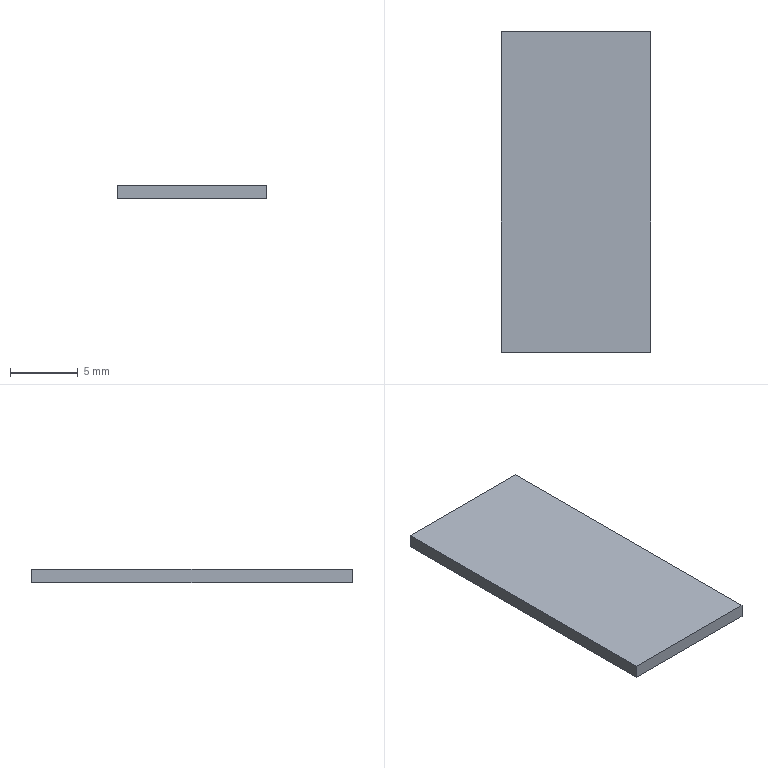Part | NX | features DATUM_CSYS 2, EXTRUDE 1, SKETCH 1 | 1 solid | 6 faces | box 11.058 x 23.696 x 1 mm | volume 262.025 mm3 | plane 6
STEP:
#1=CARTESIAN_POINT('',(-6.058,9.696,0.));
#2=VERTEX_POINT('',#1);
#3=CARTESIAN_POINT('',(-6.058,-14.,0.));
#4=VERTEX_POINT('',#3);
#5=CARTESIAN_POINT('',(-6.058,9.696,0.));
#6=DIRECTION('',(0.,-1.,0.));
#7=VECTOR('',#6,1000.);
#8=LINE('',#5,#7);
#9=EDGE_CURVE('',#2,#4,#8,.T.);
#10=ORIENTED_EDGE('',*,*,#9,.T.);
#11=CARTESIAN_POINT('',(-6.058,-14.,1.));
#12=VERTEX_POINT('',#11);
#13=CARTESIAN_POINT('',(-6.058,-14.,1.));
#14=DIRECTION('',(0.,0.,-1.));
#15=VECTOR('',#14,1000.);
#16=LINE('',#13,#15);
#17=EDGE_CURVE('',#12,#4,#16,.T.);
#18=ORIENTED_EDGE('',*,*,#17,.F.);
#19=CARTESIAN_POINT('',(-6.058,9.696,1.));
#20=VERTEX_POINT('',#19);
#21=CARTESIAN_POINT('',(-6.058,9.696,1.));
#22=DIRECTION('',(0.,-1.,0.));
#23=VECTOR('',#22,1000.);
#24=LINE('',#21,#23);
#25=EDGE_CURVE('',#20,#12,#24,.T.);
#26=ORIENTED_EDGE('',*,*,#25,.F.);
#27=CARTESIAN_POINT('',(-6.058,9.696,1.));
#28=DIRECTION('',(0.,0.,-1.));
#29=VECTOR('',#28,1000.);
#30=LINE('',#27,#29);
#31=EDGE_CURVE('',#20,#2,#30,.T.);
#32=ORIENTED_EDGE('',*,*,#31,.T.);
#33=EDGE_LOOP('',(#10,#18,#26,#32));
#34=FACE_BOUND('',#33,.T.);
#35=CARTESIAN_POINT('',(-6.058,9.696,1.));
#36=DIRECTION('',(1.,0.,0.));
#37=DIRECTION('',(0.,1.,0.));
#38=AXIS2_PLACEMENT_3D('',#35,#36,#37);
#39=PLANE('',#38);
#40=ADVANCED_FACE('',(#34),#39,.F.);
#41=CARTESIAN_POINT('',(5.,-14.,0.));
#42=VERTEX_POINT('',#41);
#43=CARTESIAN_POINT('',(-6.058,-14.,0.));
#44=DIRECTION('',(1.,0.,0.));
#45=VECTOR('',#44,1000.);
#46=LINE('',#43,#45);
#47=EDGE_CURVE('',#4,#42,#46,.T.);
#48=ORIENTED_EDGE('',*,*,#47,.T.);
#49=CARTESIAN_POINT('',(5.,-14.,1.));
#50=VERTEX_POINT('',#49);
#51=CARTESIAN_POINT('',(5.,-14.,1.));
#52=DIRECTION('',(0.,0.,-1.));
#53=VECTOR('',#52,1000.);
#54=LINE('',#51,#53);
#55=EDGE_CURVE('',#50,#42,#54,.T.);
#56=ORIENTED_EDGE('',*,*,#55,.F.);
#57=CARTESIAN_POINT('',(-6.058,-14.,1.));
#58=DIRECTION('',(1.,0.,0.));
#59=VECTOR('',#58,1000.);
#60=LINE('',#57,#59);
#61=EDGE_CURVE('',#12,#50,#60,.T.);
#62=ORIENTED_EDGE('',*,*,#61,.F.);
#63=ORIENTED_EDGE('',*,*,#17,.T.);
#64=EDGE_LOOP('',(#48,#56,#62,#63));
#65=FACE_BOUND('',#64,.T.);
#66=CARTESIAN_POINT('',(-6.058,-14.,1.));
#67=DIRECTION('',(0.,1.,0.));
#68=DIRECTION('',(-1.,0.,0.));
#69=AXIS2_PLACEMENT_3D('',#66,#67,#68);
#70=PLANE('',#69);
#71=ADVANCED_FACE('',(#65),#70,.F.);
#72=CARTESIAN_POINT('',(5.,9.696,0.));
#73=VERTEX_POINT('',#72);
#74=CARTESIAN_POINT('',(5.,-14.,0.));
#75=DIRECTION('',(0.,1.,0.));
#76=VECTOR('',#75,1000.);
#77=LINE('',#74,#76);
#78=EDGE_CURVE('',#42,#73,#77,.T.);
#79=ORIENTED_EDGE('',*,*,#78,.T.);
#80=CARTESIAN_POINT('',(5.,9.696,1.));
#81=VERTEX_POINT('',#80);
#82=CARTESIAN_POINT('',(5.,9.696,1.));
#83=DIRECTION('',(0.,0.,-1.));
#84=VECTOR('',#83,1000.);
#85=LINE('',#82,#84);
#86=EDGE_CURVE('',#81,#73,#85,.T.);
#87=ORIENTED_EDGE('',*,*,#86,.F.);
#88=CARTESIAN_POINT('',(5.,-14.,1.));
#89=DIRECTION('',(0.,1.,0.));
#90=VECTOR('',#89,1000.);
#91=LINE('',#88,#90);
#92=EDGE_CURVE('',#50,#81,#91,.T.);
#93=ORIENTED_EDGE('',*,*,#92,.F.);
#94=ORIENTED_EDGE('',*,*,#55,.T.);
#95=EDGE_LOOP('',(#79,#87,#93,#94));
#96=FACE_BOUND('',#95,.T.);
#97=CARTESIAN_POINT('',(5.,-14.,1.));
#98=DIRECTION('',(-1.,0.,0.));
#99=DIRECTION('',(0.,0.,1.));
#100=AXIS2_PLACEMENT_3D('',#97,#98,#99);
#101=PLANE('',#100);
#102=ADVANCED_FACE('',(#96),#101,.F.);
#103=CARTESIAN_POINT('',(5.,9.696,0.));
#104=DIRECTION('',(-1.,0.,0.));
#105=VECTOR('',#104,1000.);
#106=LINE('',#103,#105);
#107=EDGE_CURVE('',#73,#2,#106,.T.);
#108=ORIENTED_EDGE('',*,*,#107,.T.);
#109=ORIENTED_EDGE('',*,*,#31,.F.);
#110=CARTESIAN_POINT('',(5.,9.696,1.));
#111=DIRECTION('',(-1.,0.,0.));
#112=VECTOR('',#111,1000.);
#113=LINE('',#110,#112);
#114=EDGE_CURVE('',#81,#20,#113,.T.);
#115=ORIENTED_EDGE('',*,*,#114,.F.);
#116=ORIENTED_EDGE('',*,*,#86,.T.);
#117=EDGE_LOOP('',(#108,#109,#115,#116));
#118=FACE_BOUND('',#117,.T.);
#119=CARTESIAN_POINT('',(5.,9.696,1.));
#120=DIRECTION('',(0.,-1.,0.));
#121=DIRECTION('',(0.,0.,-1.));
#122=AXIS2_PLACEMENT_3D('',#119,#120,#121);
#123=PLANE('',#122);
#124=ADVANCED_FACE('',(#118),#123,.F.);
#125=ORIENTED_EDGE('',*,*,#25,.T.);
#126=ORIENTED_EDGE('',*,*,#61,.T.);
#127=ORIENTED_EDGE('',*,*,#92,.T.);
#128=ORIENTED_EDGE('',*,*,#114,.T.);
#129=EDGE_LOOP('',(#125,#126,#127,#128));
#130=FACE_BOUND('',#129,.T.);
#131=CARTESIAN_POINT('',(0.,0.,1.));
#132=DIRECTION('',(0.,0.,1.));
#133=DIRECTION('',(1.,0.,0.));
#134=AXIS2_PLACEMENT_3D('',#131,#132,#133);
#135=PLANE('',#134);
#136=ADVANCED_FACE('',(#130),#135,.T.);
#137=ORIENTED_EDGE('',*,*,#9,.F.);
#138=ORIENTED_EDGE('',*,*,#107,.F.);
#139=ORIENTED_EDGE('',*,*,#78,.F.);
#140=ORIENTED_EDGE('',*,*,#47,.F.);
#141=EDGE_LOOP('',(#137,#138,#139,#140));
#142=FACE_BOUND('',#141,.T.);
#143=CARTESIAN_POINT('',(0.,0.,0.));
#144=DIRECTION('',(0.,0.,1.));
#145=DIRECTION('',(1.,0.,0.));
#146=AXIS2_PLACEMENT_3D('',#143,#144,#145);
#147=PLANE('',#146);
#148=ADVANCED_FACE('',(#142),#147,.F.);
#149=CLOSED_SHELL('',(#40,#71,#102,#124,#136,#148));
#150=MANIFOLD_SOLID_BREP('',#149);
#151=(LENGTH_UNIT()NAMED_UNIT(*)SI_UNIT(.MILLI.,.METRE.));
#152=UNCERTAINTY_MEASURE_WITH_UNIT(LENGTH_MEASURE(0.00001),#151,'','');
#153=(NAMED_UNIT(*)PLANE_ANGLE_UNIT()SI_UNIT($,.RADIAN.));
#154=(NAMED_UNIT(*)SI_UNIT($,.STERADIAN.)SOLID_ANGLE_UNIT());
#155=(GEOMETRIC_REPRESENTATION_CONTEXT(3)GLOBAL_UNCERTAINTY_ASSIGNED_CONTEXT((#152))GLOBAL_UNIT_ASSIGNED_CONTEXT((#151,#153,#154))REPRESENTATION_CONTEXT('',''));
#156=ADVANCED_BREP_SHAPE_REPRESENTATION('',(#150),#155);